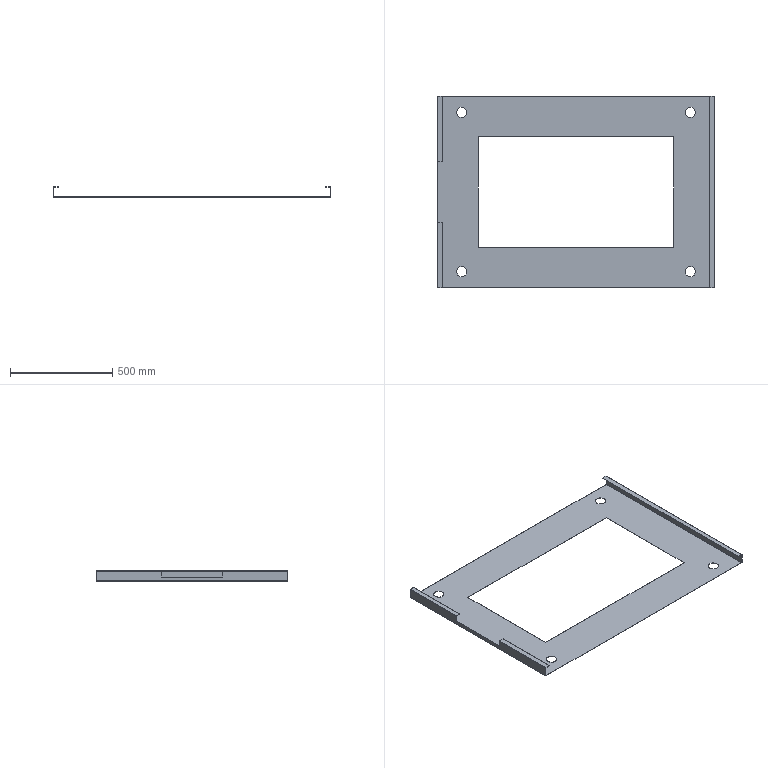Part | SolidWorks | features Cut 4, EdgeFlange 2, FlatPattern 1, ICE 1, SMBaseFlange 1, SheetMetal 1 | 1 solid | 62 faces | box 1360 x 940 x 50 mm | volume 873442 mm3 | plane 44 | cylinder 18 | commonest cylinder face diameters 50 x8 0.4 x5 2.4 x5